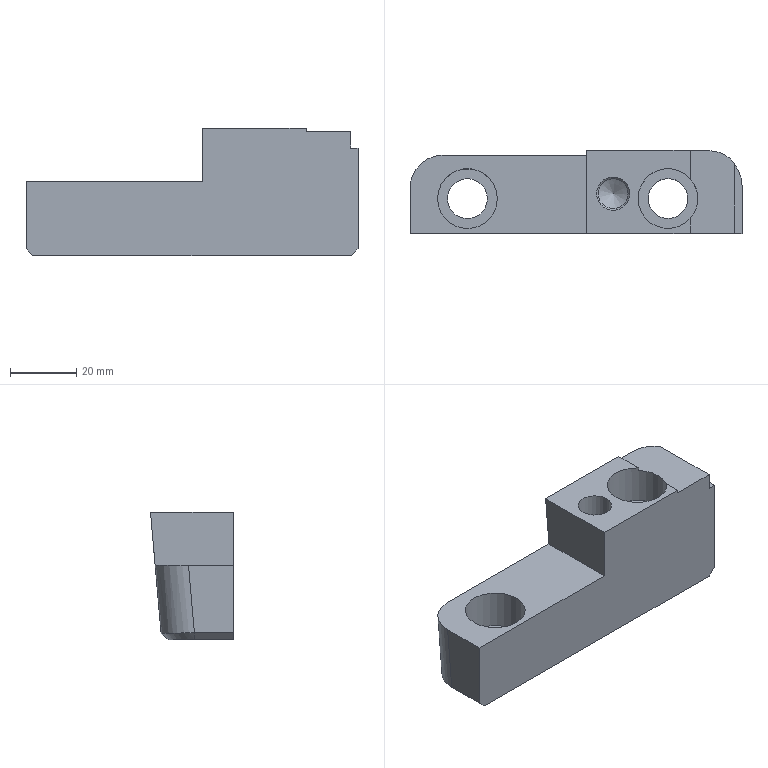Part | STEP file | solid 78 | 1 solid | 30 faces | box 100 x 25 x 38.403 mm | volume 54742 mm3 | plane 18 | cylinder 8 | spline 2 | cone 2 | commonest cylinder face diameters 12 x2 18 x2 20 x2 9 x1 10 x1